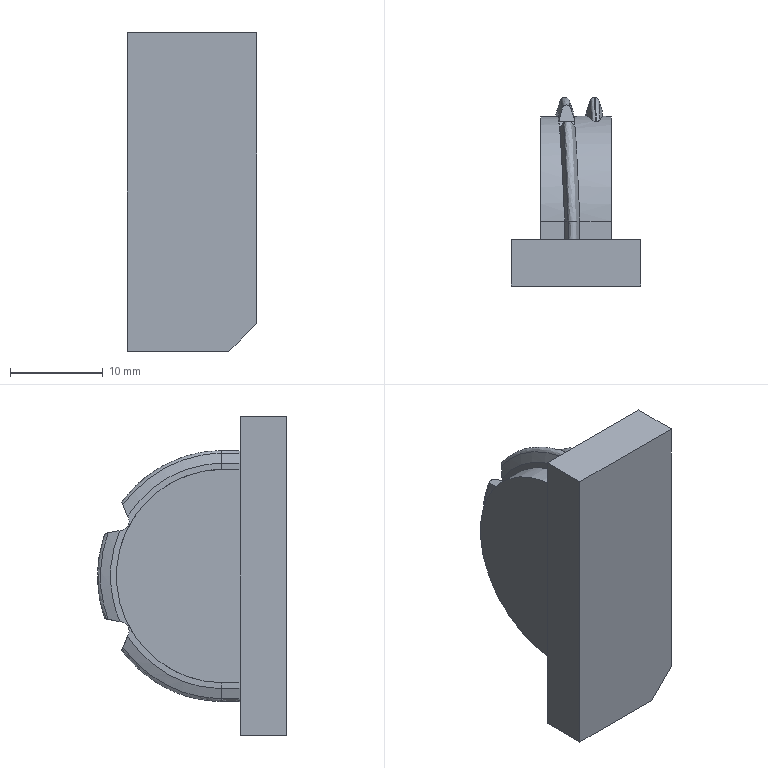Part | 1 solid | 58 faces | box 13.933 x 20.347 x 34.335 mm | volume 4427 mm3 | spline 27 | plane 26 | cylinder 5 | commonest cylinder face diameters 1.9 x3 22.985 x2